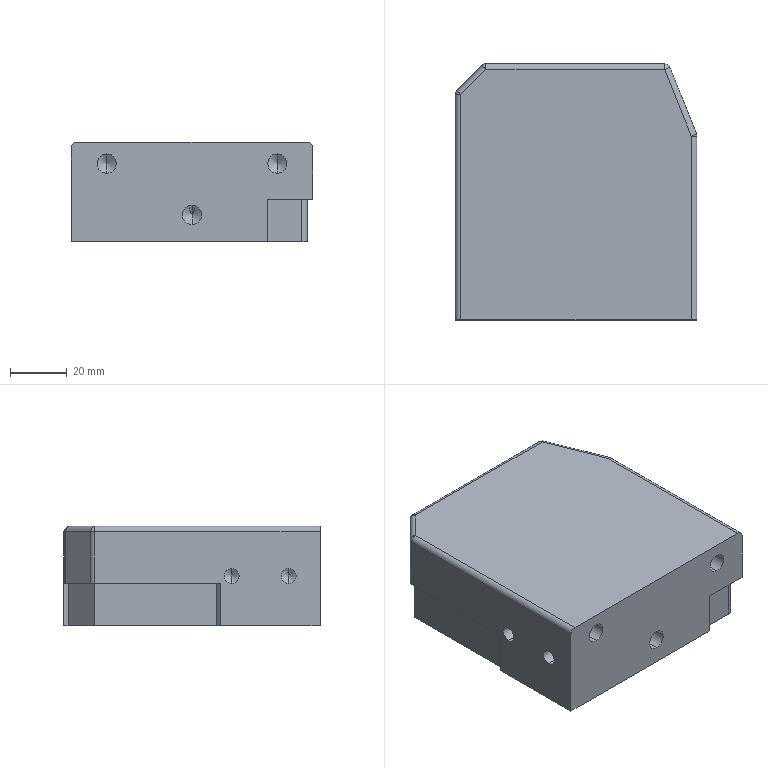Part | STEP file | Guide rail stopper 2 | 1 solid | 59 faces | box 85 x 90 x 35 mm | volume 251196 mm3 | cylinder 23 | plane 22 | cone 10 | sphere 4 | commonest cylinder face diameters 4 x13 6.8 x6 5.25 x4